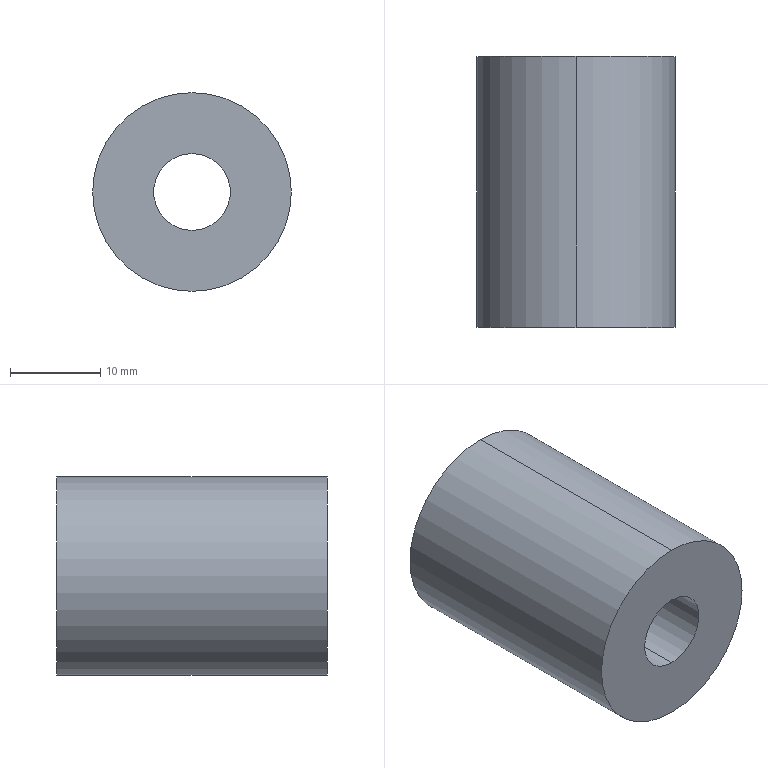Part | SolidWorks | features Extrusion 1, HoleWzd 1 | 1 solid | 6 faces | box 22 x 30 x 22 mm | volume 9702 mm3 | cylinder 4 | plane 2 | commonest cylinder face diameters 8.5 x2 22 x2
STEP:
#1=CARTESIAN_POINT('',(0.,0.,-4.25));
#2=VERTEX_POINT('',#1);
#3=CARTESIAN_POINT('',(0.,0.,4.25));
#4=VERTEX_POINT('',#3);
#5=CARTESIAN_POINT('',(0.,0.,0.));
#6=DIRECTION('',(0.,1.,0.));
#7=DIRECTION('',(0.,0.,1.));
#8=AXIS2_PLACEMENT_3D('',#5,#6,#7);
#9=CIRCLE('',#8,4.25);
#10=EDGE_CURVE('',#2,#4,#9,.T.);
#11=ORIENTED_EDGE('',*,*,#10,.F.);
#12=CARTESIAN_POINT('',(0.,30.,-4.25));
#13=VERTEX_POINT('',#12);
#14=CARTESIAN_POINT('',(0.,30.,-4.25));
#15=DIRECTION('',(0.,1.,0.));
#16=VECTOR('',#15,1000.);
#17=LINE('',#14,#16);
#18=EDGE_CURVE('',#2,#13,#17,.T.);
#19=ORIENTED_EDGE('',*,*,#18,.T.);
#20=CARTESIAN_POINT('',(0.,30.,4.25));
#21=VERTEX_POINT('',#20);
#22=CARTESIAN_POINT('',(0.,30.,0.));
#23=DIRECTION('',(0.,1.,0.));
#24=DIRECTION('',(0.,0.,1.));
#25=AXIS2_PLACEMENT_3D('',#22,#23,#24);
#26=CIRCLE('',#25,4.25);
#27=EDGE_CURVE('',#13,#21,#26,.T.);
#28=ORIENTED_EDGE('',*,*,#27,.T.);
#29=CARTESIAN_POINT('',(0.,30.,4.25));
#30=DIRECTION('',(0.,1.,0.));
#31=VECTOR('',#30,1000.);
#32=LINE('',#29,#31);
#33=EDGE_CURVE('',#4,#21,#32,.T.);
#34=ORIENTED_EDGE('',*,*,#33,.F.);
#35=EDGE_LOOP('',(#11,#19,#28,#34));
#36=FACE_OUTER_BOUND('',#35,.T.);
#37=CARTESIAN_POINT('',(0.,30.,0.));
#38=DIRECTION('',(0.,1.,0.));
#39=DIRECTION('',(0.,0.,1.));
#40=AXIS2_PLACEMENT_3D('',#37,#38,#39);
#41=CYLINDRICAL_SURFACE('',#40,4.25);
#42=ADVANCED_FACE('',(#36),#41,.F.);
#43=CARTESIAN_POINT('',(0.,30.,11.));
#44=VERTEX_POINT('',#43);
#45=CARTESIAN_POINT('',(0.,30.,-11.));
#46=VERTEX_POINT('',#45);
#47=CARTESIAN_POINT('',(0.,30.,0.));
#48=DIRECTION('',(0.,1.,0.));
#49=DIRECTION('',(0.,0.,1.));
#50=AXIS2_PLACEMENT_3D('',#47,#48,#49);
#51=CIRCLE('',#50,11.);
#52=EDGE_CURVE('',#44,#46,#51,.T.);
#53=ORIENTED_EDGE('',*,*,#52,.F.);
#54=CARTESIAN_POINT('',(0.,0.,11.));
#55=VERTEX_POINT('',#54);
#56=CARTESIAN_POINT('',(0.,30.,11.));
#57=DIRECTION('',(0.,-1.,0.));
#58=VECTOR('',#57,1000.);
#59=LINE('',#56,#58);
#60=EDGE_CURVE('',#44,#55,#59,.T.);
#61=ORIENTED_EDGE('',*,*,#60,.T.);
#62=CARTESIAN_POINT('',(0.,0.,-11.));
#63=VERTEX_POINT('',#62);
#64=CARTESIAN_POINT('',(0.,0.,0.));
#65=DIRECTION('',(0.,1.,0.));
#66=DIRECTION('',(0.,0.,1.));
#67=AXIS2_PLACEMENT_3D('',#64,#65,#66);
#68=CIRCLE('',#67,11.);
#69=EDGE_CURVE('',#55,#63,#68,.T.);
#70=ORIENTED_EDGE('',*,*,#69,.T.);
#71=CARTESIAN_POINT('',(0.,30.,-11.));
#72=DIRECTION('',(0.,-1.,0.));
#73=VECTOR('',#72,1000.);
#74=LINE('',#71,#73);
#75=EDGE_CURVE('',#46,#63,#74,.T.);
#76=ORIENTED_EDGE('',*,*,#75,.F.);
#77=EDGE_LOOP('',(#53,#61,#70,#76));
#78=FACE_OUTER_BOUND('',#77,.T.);
#79=CARTESIAN_POINT('',(0.,30.,0.));
#80=DIRECTION('',(0.,-1.,0.));
#81=DIRECTION('',(0.,0.,-1.));
#82=AXIS2_PLACEMENT_3D('',#79,#80,#81);
#83=CYLINDRICAL_SURFACE('',#82,11.);
#84=ADVANCED_FACE('',(#78),#83,.T.);
#85=ORIENTED_EDGE('',*,*,#60,.F.);
#86=CARTESIAN_POINT('',(0.,30.,0.));
#87=DIRECTION('',(0.,1.,0.));
#88=DIRECTION('',(0.,0.,1.));
#89=AXIS2_PLACEMENT_3D('',#86,#87,#88);
#90=CIRCLE('',#89,11.);
#91=EDGE_CURVE('',#46,#44,#90,.T.);
#92=ORIENTED_EDGE('',*,*,#91,.F.);
#93=ORIENTED_EDGE('',*,*,#75,.T.);
#94=CARTESIAN_POINT('',(0.,0.,0.));
#95=DIRECTION('',(0.,1.,0.));
#96=DIRECTION('',(0.,0.,1.));
#97=AXIS2_PLACEMENT_3D('',#94,#95,#96);
#98=CIRCLE('',#97,11.);
#99=EDGE_CURVE('',#63,#55,#98,.T.);
#100=ORIENTED_EDGE('',*,*,#99,.T.);
#101=EDGE_LOOP('',(#85,#92,#93,#100));
#102=FACE_OUTER_BOUND('',#101,.T.);
#103=CARTESIAN_POINT('',(0.,30.,0.));
#104=DIRECTION('',(0.,-1.,0.));
#105=DIRECTION('',(0.,0.,-1.));
#106=AXIS2_PLACEMENT_3D('',#103,#104,#105);
#107=CYLINDRICAL_SURFACE('',#106,11.);
#108=ADVANCED_FACE('',(#102),#107,.T.);
#109=CARTESIAN_POINT('',(0.,30.,0.));
#110=DIRECTION('',(0.,1.,0.));
#111=DIRECTION('',(0.,0.,1.));
#112=AXIS2_PLACEMENT_3D('',#109,#110,#111);
#113=CIRCLE('',#112,4.25);
#114=EDGE_CURVE('',#21,#13,#113,.T.);
#115=ORIENTED_EDGE('',*,*,#114,.F.);
#116=ORIENTED_EDGE('',*,*,#27,.F.);
#117=EDGE_LOOP('',(#115,#116));
#118=FACE_BOUND('',#117,.T.);
#119=ORIENTED_EDGE('',*,*,#91,.T.);
#120=ORIENTED_EDGE('',*,*,#52,.T.);
#121=EDGE_LOOP('',(#119,#120));
#122=FACE_OUTER_BOUND('',#121,.T.);
#123=CARTESIAN_POINT('',(0.,30.,0.));
#124=DIRECTION('',(0.,1.,0.));
#125=DIRECTION('',(0.,0.,1.));
#126=AXIS2_PLACEMENT_3D('',#123,#124,#125);
#127=PLANE('',#126);
#128=ADVANCED_FACE('',(#118,#122),#127,.T.);
#129=CARTESIAN_POINT('',(0.,0.,0.));
#130=DIRECTION('',(0.,1.,0.));
#131=DIRECTION('',(0.,0.,1.));
#132=AXIS2_PLACEMENT_3D('',#129,#130,#131);
#133=CIRCLE('',#132,4.25);
#134=EDGE_CURVE('',#4,#2,#133,.T.);
#135=ORIENTED_EDGE('',*,*,#134,.T.);
#136=ORIENTED_EDGE('',*,*,#10,.T.);
#137=EDGE_LOOP('',(#135,#136));
#138=FACE_BOUND('',#137,.T.);
#139=ORIENTED_EDGE('',*,*,#99,.F.);
#140=ORIENTED_EDGE('',*,*,#69,.F.);
#141=EDGE_LOOP('',(#139,#140));
#142=FACE_OUTER_BOUND('',#141,.T.);
#143=CARTESIAN_POINT('',(0.,0.,0.));
#144=DIRECTION('',(0.,1.,0.));
#145=DIRECTION('',(0.,0.,1.));
#146=AXIS2_PLACEMENT_3D('',#143,#144,#145);
#147=PLANE('',#146);
#148=ADVANCED_FACE('',(#138,#142),#147,.F.);
#149=ORIENTED_EDGE('',*,*,#18,.F.);
#150=ORIENTED_EDGE('',*,*,#134,.F.);
#151=ORIENTED_EDGE('',*,*,#33,.T.);
#152=ORIENTED_EDGE('',*,*,#114,.T.);
#153=EDGE_LOOP('',(#149,#150,#151,#152));
#154=FACE_OUTER_BOUND('',#153,.T.);
#155=CARTESIAN_POINT('',(0.,30.,0.));
#156=DIRECTION('',(0.,1.,0.));
#157=DIRECTION('',(0.,0.,1.));
#158=AXIS2_PLACEMENT_3D('',#155,#156,#157);
#159=CYLINDRICAL_SURFACE('',#158,4.25);
#160=ADVANCED_FACE('',(#154),#159,.F.);
#161=CLOSED_SHELL('',(#42,#84,#108,#128,#148,#160));
#162=MANIFOLD_SOLID_BREP('',#161);
#163=CARTESIAN_POINT('',(0.,0.,0.));
#164=DIRECTION('',(0.,0.,1.));
#165=DIRECTION('',(1.,0.,0.));
#166=AXIS2_PLACEMENT_3D('',#163,#164,#165);
#167=(LENGTH_UNIT()NAMED_UNIT(*)SI_UNIT(.MILLI.,.METRE.));
#168=UNCERTAINTY_MEASURE_WITH_UNIT(LENGTH_MEASURE(0.00001),#167,'','');
#169=(NAMED_UNIT(*)PLANE_ANGLE_UNIT()SI_UNIT($,.RADIAN.));
#170=(NAMED_UNIT(*)SI_UNIT($,.STERADIAN.)SOLID_ANGLE_UNIT());
#171=(GEOMETRIC_REPRESENTATION_CONTEXT(3)GLOBAL_UNCERTAINTY_ASSIGNED_CONTEXT((#168))GLOBAL_UNIT_ASSIGNED_CONTEXT((#167,#169,#170))REPRESENTATION_CONTEXT('',''));
#172=ADVANCED_BREP_SHAPE_REPRESENTATION('',(#162,#166),#171);